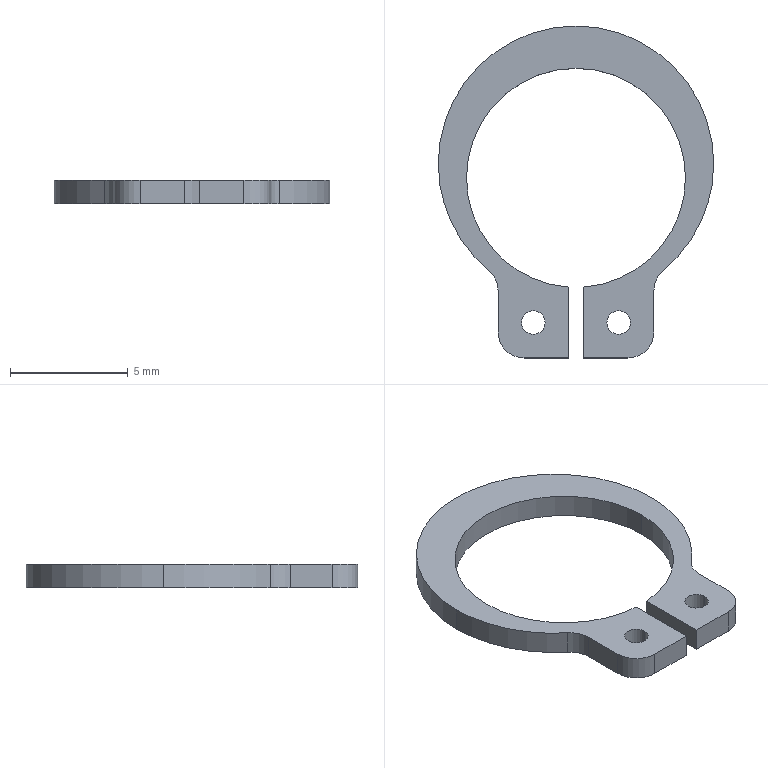Part | NX | features BREP 1 | 1 solid | 22 faces | box 11.7 x 14.1 x 1 mm | volume 53.779 mm3 | cylinder 14 | plane 8 | commonest cylinder face diameters 1 x4 2.207 x4 9.3 x3 11.7 x3
STEP:
#1=CARTESIAN_POINT('',(-2.31,-6.15,0.5));
#2=VERTEX_POINT('',#1);
#3=CARTESIAN_POINT('',(-1.31,-6.15,0.5));
#4=VERTEX_POINT('',#3);
#5=CARTESIAN_POINT('',(-1.81,-6.15,0.5));
#6=DIRECTION('',(0.,0.,1.));
#7=DIRECTION('',(1.,0.,0.));
#8=AXIS2_PLACEMENT_3D('',#5,#6,#7);
#9=CIRCLE('',#8,0.5);
#10=EDGE_CURVE('',#2,#4,#9,.T.);
#11=ORIENTED_EDGE('',*,*,#10,.T.);
#12=CARTESIAN_POINT('',(-1.31,-6.15,-0.5));
#13=VERTEX_POINT('',#12);
#14=CARTESIAN_POINT('',(-1.31,-6.15,0.5));
#15=DIRECTION('',(0.,0.,-1.));
#16=VECTOR('',#15,1000.);
#17=LINE('',#14,#16);
#18=EDGE_CURVE('',#13,#4,#17,.F.);
#19=ORIENTED_EDGE('',*,*,#18,.F.);
#20=CARTESIAN_POINT('',(-2.31,-6.15,-0.5));
#21=VERTEX_POINT('',#20);
#22=CARTESIAN_POINT('',(-1.81,-6.15,-0.5));
#23=DIRECTION('',(0.,0.,1.));
#24=DIRECTION('',(1.,0.,0.));
#25=AXIS2_PLACEMENT_3D('',#22,#23,#24);
#26=CIRCLE('',#25,0.5);
#27=EDGE_CURVE('',#21,#13,#26,.T.);
#28=ORIENTED_EDGE('',*,*,#27,.F.);
#29=CARTESIAN_POINT('',(-2.31,-6.15,0.5));
#30=DIRECTION('',(0.,0.,-1.));
#31=VECTOR('',#30,1000.);
#32=LINE('',#29,#31);
#33=EDGE_CURVE('',#21,#2,#32,.F.);
#34=ORIENTED_EDGE('',*,*,#33,.T.);
#35=EDGE_LOOP('',(#11,#19,#28,#34));
#36=FACE_BOUND('',#35,.T.);
#37=CARTESIAN_POINT('',(-1.81,-6.15,0.5));
#38=DIRECTION('',(0.,0.,-1.));
#39=DIRECTION('',(1.,0.,0.));
#40=AXIS2_PLACEMENT_3D('',#37,#38,#39);
#41=CYLINDRICAL_SURFACE('',#40,0.5);
#42=ADVANCED_FACE('',(#36),#41,.F.);
#43=CARTESIAN_POINT('',(1.31,-6.15,0.5));
#44=VERTEX_POINT('',#43);
#45=CARTESIAN_POINT('',(2.31,-6.15,0.5));
#46=VERTEX_POINT('',#45);
#47=CARTESIAN_POINT('',(1.81,-6.15,0.5));
#48=DIRECTION('',(0.,0.,1.));
#49=DIRECTION('',(1.,0.,0.));
#50=AXIS2_PLACEMENT_3D('',#47,#48,#49);
#51=CIRCLE('',#50,0.5);
#52=EDGE_CURVE('',#44,#46,#51,.T.);
#53=ORIENTED_EDGE('',*,*,#52,.T.);
#54=CARTESIAN_POINT('',(2.31,-6.15,-0.5));
#55=VERTEX_POINT('',#54);
#56=CARTESIAN_POINT('',(2.31,-6.15,0.5));
#57=DIRECTION('',(0.,0.,-1.));
#58=VECTOR('',#57,1000.);
#59=LINE('',#56,#58);
#60=EDGE_CURVE('',#55,#46,#59,.F.);
#61=ORIENTED_EDGE('',*,*,#60,.F.);
#62=CARTESIAN_POINT('',(1.31,-6.15,-0.5));
#63=VERTEX_POINT('',#62);
#64=CARTESIAN_POINT('',(1.81,-6.15,-0.5));
#65=DIRECTION('',(0.,0.,1.));
#66=DIRECTION('',(1.,0.,0.));
#67=AXIS2_PLACEMENT_3D('',#64,#65,#66);
#68=CIRCLE('',#67,0.5);
#69=EDGE_CURVE('',#63,#55,#68,.T.);
#70=ORIENTED_EDGE('',*,*,#69,.F.);
#71=CARTESIAN_POINT('',(1.31,-6.15,0.5));
#72=DIRECTION('',(0.,0.,-1.));
#73=VECTOR('',#72,1000.);
#74=LINE('',#71,#73);
#75=EDGE_CURVE('',#63,#44,#74,.F.);
#76=ORIENTED_EDGE('',*,*,#75,.T.);
#77=EDGE_LOOP('',(#53,#61,#70,#76));
#78=FACE_BOUND('',#77,.T.);
#79=CARTESIAN_POINT('',(1.81,-6.15,0.5));
#80=DIRECTION('',(0.,0.,-1.));
#81=DIRECTION('',(1.,0.,0.));
#82=AXIS2_PLACEMENT_3D('',#79,#80,#81);
#83=CYLINDRICAL_SURFACE('',#82,0.5);
#84=ADVANCED_FACE('',(#78),#83,.F.);
#85=CARTESIAN_POINT('',(4.65,0.,0.5));
#86=VERTEX_POINT('',#85);
#87=CARTESIAN_POINT('',(0.31,-4.64,0.5));
#88=VERTEX_POINT('',#87);
#89=CARTESIAN_POINT('',(0.,0.,0.5));
#90=DIRECTION('',(0.,0.,-1.));
#91=DIRECTION('',(-1.,0.,0.));
#92=AXIS2_PLACEMENT_3D('',#89,#90,#91);
#93=CIRCLE('',#92,4.65);
#94=EDGE_CURVE('',#86,#88,#93,.T.);
#95=ORIENTED_EDGE('',*,*,#94,.F.);
#96=CARTESIAN_POINT('',(4.65,0.,-0.5));
#97=VERTEX_POINT('',#96);
#98=CARTESIAN_POINT('',(4.65,0.,0.5));
#99=DIRECTION('',(0.,0.,-1.));
#100=VECTOR('',#99,1000.);
#101=LINE('',#98,#100);
#102=EDGE_CURVE('',#86,#97,#101,.T.);
#103=ORIENTED_EDGE('',*,*,#102,.T.);
#104=CARTESIAN_POINT('',(0.31,-4.64,-0.5));
#105=VERTEX_POINT('',#104);
#106=CARTESIAN_POINT('',(0.,0.,-0.5));
#107=DIRECTION('',(0.,0.,-1.));
#108=DIRECTION('',(-1.,0.,0.));
#109=AXIS2_PLACEMENT_3D('',#106,#107,#108);
#110=CIRCLE('',#109,4.65);
#111=EDGE_CURVE('',#97,#105,#110,.T.);
#112=ORIENTED_EDGE('',*,*,#111,.T.);
#113=CARTESIAN_POINT('',(0.31,-4.64,0.5));
#114=DIRECTION('',(0.,0.,-1.));
#115=VECTOR('',#114,1000.);
#116=LINE('',#113,#115);
#117=EDGE_CURVE('',#88,#105,#116,.T.);
#118=ORIENTED_EDGE('',*,*,#117,.F.);
#119=EDGE_LOOP('',(#95,#103,#112,#118));
#120=FACE_BOUND('',#119,.T.);
#121=CARTESIAN_POINT('',(0.,0.,0.5));
#122=DIRECTION('',(0.,0.,-1.));
#123=DIRECTION('',(1.,0.,0.));
#124=AXIS2_PLACEMENT_3D('',#121,#122,#123);
#125=CYLINDRICAL_SURFACE('',#124,4.65);
#126=ADVANCED_FACE('',(#120),#125,.F.);
#127=ORIENTED_EDGE('',*,*,#102,.F.);
#128=CARTESIAN_POINT('',(-4.65,0.,0.5));
#129=VERTEX_POINT('',#128);
#130=CARTESIAN_POINT('',(0.,0.,0.5));
#131=DIRECTION('',(0.,0.,-1.));
#132=DIRECTION('',(-1.,0.,0.));
#133=AXIS2_PLACEMENT_3D('',#130,#131,#132);
#134=CIRCLE('',#133,4.65);
#135=EDGE_CURVE('',#129,#86,#134,.T.);
#136=ORIENTED_EDGE('',*,*,#135,.F.);
#137=CARTESIAN_POINT('',(-4.65,0.,-0.5));
#138=VERTEX_POINT('',#137);
#139=CARTESIAN_POINT('',(-4.65,0.,0.5));
#140=DIRECTION('',(0.,0.,-1.));
#141=VECTOR('',#140,1000.);
#142=LINE('',#139,#141);
#143=EDGE_CURVE('',#129,#138,#142,.T.);
#144=ORIENTED_EDGE('',*,*,#143,.T.);
#145=CARTESIAN_POINT('',(0.,0.,-0.5));
#146=DIRECTION('',(0.,0.,-1.));
#147=DIRECTION('',(-1.,0.,0.));
#148=AXIS2_PLACEMENT_3D('',#145,#146,#147);
#149=CIRCLE('',#148,4.65);
#150=EDGE_CURVE('',#138,#97,#149,.T.);
#151=ORIENTED_EDGE('',*,*,#150,.T.);
#152=EDGE_LOOP('',(#127,#136,#144,#151));
#153=FACE_BOUND('',#152,.T.);
#154=CARTESIAN_POINT('',(0.,0.,0.5));
#155=DIRECTION('',(0.,0.,-1.));
#156=DIRECTION('',(1.,0.,0.));
#157=AXIS2_PLACEMENT_3D('',#154,#155,#156);
#158=CYLINDRICAL_SURFACE('',#157,4.65);
#159=ADVANCED_FACE('',(#153),#158,.F.);
#160=CARTESIAN_POINT('',(5.85,0.6,0.5));
#161=VERTEX_POINT('',#160);
#162=CARTESIAN_POINT('',(-5.85,0.6,0.5));
#163=VERTEX_POINT('',#162);
#164=CARTESIAN_POINT('',(0.,0.6,0.5));
#165=DIRECTION('',(0.,0.,1.));
#166=DIRECTION('',(1.,0.,0.));
#167=AXIS2_PLACEMENT_3D('',#164,#165,#166);
#168=CIRCLE('',#167,5.85);
#169=EDGE_CURVE('',#161,#163,#168,.T.);
#170=ORIENTED_EDGE('',*,*,#169,.F.);
#171=CARTESIAN_POINT('',(5.85,0.6,-0.5));
#172=VERTEX_POINT('',#171);
#173=CARTESIAN_POINT('',(5.85,0.6,0.5));
#174=DIRECTION('',(0.,0.,-1.));
#175=VECTOR('',#174,1000.);
#176=LINE('',#173,#175);
#177=EDGE_CURVE('',#161,#172,#176,.T.);
#178=ORIENTED_EDGE('',*,*,#177,.T.);
#179=CARTESIAN_POINT('',(-5.85,0.6,-0.5));
#180=VERTEX_POINT('',#179);
#181=CARTESIAN_POINT('',(0.,0.6,-0.5));
#182=DIRECTION('',(0.,0.,1.));
#183=DIRECTION('',(1.,0.,0.));
#184=AXIS2_PLACEMENT_3D('',#181,#182,#183);
#185=CIRCLE('',#184,5.85);
#186=EDGE_CURVE('',#172,#180,#185,.T.);
#187=ORIENTED_EDGE('',*,*,#186,.T.);
#188=CARTESIAN_POINT('',(-5.85,0.6,0.5));
#189=DIRECTION('',(0.,0.,-1.));
#190=VECTOR('',#189,1000.);
#191=LINE('',#188,#190);
#192=EDGE_CURVE('',#163,#180,#191,.T.);
#193=ORIENTED_EDGE('',*,*,#192,.F.);
#194=EDGE_LOOP('',(#170,#178,#187,#193));
#195=FACE_BOUND('',#194,.T.);
#196=CARTESIAN_POINT('',(0.,0.6,0.5));
#197=DIRECTION('',(0.,0.,-1.));
#198=DIRECTION('',(1.,0.,0.));
#199=AXIS2_PLACEMENT_3D('',#196,#197,#198);
#200=CYLINDRICAL_SURFACE('',#199,5.85);
#201=ADVANCED_FACE('',(#195),#200,.T.);
#202=CARTESIAN_POINT('',(-3.713,-3.921,0.5));
#203=VERTEX_POINT('',#202);
#204=CARTESIAN_POINT('',(0.,0.6,0.5));
#205=DIRECTION('',(0.,0.,1.));
#206=DIRECTION('',(1.,0.,0.));
#207=AXIS2_PLACEMENT_3D('',#204,#205,#206);
#208=CIRCLE('',#207,5.85);
#209=EDGE_CURVE('',#163,#203,#208,.T.);
#210=ORIENTED_EDGE('',*,*,#209,.F.);
#211=ORIENTED_EDGE('',*,*,#192,.T.);
#212=CARTESIAN_POINT('',(-3.713,-3.921,-0.5));
#213=VERTEX_POINT('',#212);
#214=CARTESIAN_POINT('',(0.,0.6,-0.5));
#215=DIRECTION('',(0.,0.,1.));
#216=DIRECTION('',(1.,0.,0.));
#217=AXIS2_PLACEMENT_3D('',#214,#215,#216);
#218=CIRCLE('',#217,5.85);
#219=EDGE_CURVE('',#180,#213,#218,.T.);
#220=ORIENTED_EDGE('',*,*,#219,.T.);
#221=CARTESIAN_POINT('',(-3.713,-3.921,0.5));
#222=DIRECTION('',(0.,0.,-1.));
#223=VECTOR('',#222,1000.);
#224=LINE('',#221,#223);
#225=EDGE_CURVE('',#203,#213,#224,.T.);
#226=ORIENTED_EDGE('',*,*,#225,.F.);
#227=EDGE_LOOP('',(#210,#211,#220,#226));
#228=FACE_BOUND('',#227,.T.);
#229=CARTESIAN_POINT('',(0.,0.6,0.5));
#230=DIRECTION('',(0.,0.,-1.));
#231=DIRECTION('',(1.,0.,0.));
#232=AXIS2_PLACEMENT_3D('',#229,#230,#231);
#233=CYLINDRICAL_SURFACE('',#232,5.85);
#234=ADVANCED_FACE('',(#228),#233,.T.);
#235=CARTESIAN_POINT('',(3.31,-4.773,0.5));
#236=VERTEX_POINT('',#235);
#237=CARTESIAN_POINT('',(3.713,-3.921,0.5));
#238=VERTEX_POINT('',#237);
#239=CARTESIAN_POINT('',(4.413,-4.773,0.5));
#240=DIRECTION('',(0.,0.,-1.));
#241=DIRECTION('',(-1.,0.,0.));
#242=AXIS2_PLACEMENT_3D('',#239,#240,#241);
#243=CIRCLE('',#242,1.103);
#244=EDGE_CURVE('',#236,#238,#243,.T.);
#245=ORIENTED_EDGE('',*,*,#244,.T.);
#246=CARTESIAN_POINT('',(0.,0.6,0.5));
#247=DIRECTION('',(0.,0.,1.));
#248=DIRECTION('',(1.,0.,0.));
#249=AXIS2_PLACEMENT_3D('',#246,#247,#248);
#250=CIRCLE('',#249,5.85);
#251=EDGE_CURVE('',#238,#161,#250,.T.);
#252=ORIENTED_EDGE('',*,*,#251,.T.);
#253=ORIENTED_EDGE('',*,*,#169,.T.);
#254=ORIENTED_EDGE('',*,*,#209,.T.);
#255=CARTESIAN_POINT('',(-3.31,-4.773,0.5));
#256=VERTEX_POINT('',#255);
#257=CARTESIAN_POINT('',(-4.413,-4.773,0.5));
#258=DIRECTION('',(0.,0.,-1.));
#259=DIRECTION('',(-1.,0.,0.));
#260=AXIS2_PLACEMENT_3D('',#257,#258,#259);
#261=CIRCLE('',#260,1.103);
#262=EDGE_CURVE('',#203,#256,#261,.T.);
#263=ORIENTED_EDGE('',*,*,#262,.T.);
#264=CARTESIAN_POINT('',(-3.31,-6.547,0.5));
#265=VERTEX_POINT('',#264);
#266=CARTESIAN_POINT('',(-3.31,-4.773,0.5));
#267=DIRECTION('',(0.,-1.,0.));
#268=VECTOR('',#267,1000.);
#269=LINE('',#266,#268);
#270=EDGE_CURVE('',#256,#265,#269,.T.);
#271=ORIENTED_EDGE('',*,*,#270,.T.);
#272=CARTESIAN_POINT('',(-2.207,-7.65,0.5));
#273=VERTEX_POINT('',#272);
#274=CARTESIAN_POINT('',(-2.207,-6.547,0.5));
#275=DIRECTION('',(0.,0.,1.));
#276=DIRECTION('',(1.,0.,0.));
#277=AXIS2_PLACEMENT_3D('',#274,#275,#276);
#278=CIRCLE('',#277,1.103);
#279=EDGE_CURVE('',#265,#273,#278,.T.);
#280=ORIENTED_EDGE('',*,*,#279,.T.);
#281=CARTESIAN_POINT('',(-0.31,-7.65,0.5));
#282=VERTEX_POINT('',#281);
#283=CARTESIAN_POINT('',(-2.207,-7.65,0.5));
#284=DIRECTION('',(1.,0.,0.));
#285=VECTOR('',#284,1000.);
#286=LINE('',#283,#285);
#287=EDGE_CURVE('',#273,#282,#286,.T.);
#288=ORIENTED_EDGE('',*,*,#287,.T.);
#289=CARTESIAN_POINT('',(-0.31,-4.64,0.5));
#290=VERTEX_POINT('',#289);
#291=CARTESIAN_POINT('',(-0.31,-7.65,0.5));
#292=DIRECTION('',(0.,1.,0.));
#293=VECTOR('',#292,1000.);
#294=LINE('',#291,#293);
#295=EDGE_CURVE('',#282,#290,#294,.T.);
#296=ORIENTED_EDGE('',*,*,#295,.T.);
#297=CARTESIAN_POINT('',(0.,0.,0.5));
#298=DIRECTION('',(0.,0.,-1.));
#299=DIRECTION('',(-1.,0.,0.));
#300=AXIS2_PLACEMENT_3D('',#297,#298,#299);
#301=CIRCLE('',#300,4.65);
#302=EDGE_CURVE('',#290,#129,#301,.T.);
#303=ORIENTED_EDGE('',*,*,#302,.T.);
#304=ORIENTED_EDGE('',*,*,#135,.T.);
#305=ORIENTED_EDGE('',*,*,#94,.T.);
#306=CARTESIAN_POINT('',(0.31,-7.65,0.5));
#307=VERTEX_POINT('',#306);
#308=CARTESIAN_POINT('',(0.31,-4.64,0.5));
#309=DIRECTION('',(0.,-1.,0.));
#310=VECTOR('',#309,1000.);
#311=LINE('',#308,#310);
#312=EDGE_CURVE('',#88,#307,#311,.T.);
#313=ORIENTED_EDGE('',*,*,#312,.T.);
#314=CARTESIAN_POINT('',(2.207,-7.65,0.5));
#315=VERTEX_POINT('',#314);
#316=CARTESIAN_POINT('',(0.31,-7.65,0.5));
#317=DIRECTION('',(1.,0.,0.));
#318=VECTOR('',#317,1000.);
#319=LINE('',#316,#318);
#320=EDGE_CURVE('',#307,#315,#319,.T.);
#321=ORIENTED_EDGE('',*,*,#320,.T.);
#322=CARTESIAN_POINT('',(3.31,-6.547,0.5));
#323=VERTEX_POINT('',#322);
#324=CARTESIAN_POINT('',(2.207,-6.547,0.5));
#325=DIRECTION('',(0.,0.,1.));
#326=DIRECTION('',(1.,0.,0.));
#327=AXIS2_PLACEMENT_3D('',#324,#325,#326);
#328=CIRCLE('',#327,1.103);
#329=EDGE_CURVE('',#315,#323,#328,.T.);
#330=ORIENTED_EDGE('',*,*,#329,.T.);
#331=CARTESIAN_POINT('',(3.31,-6.547,0.5));
#332=DIRECTION('',(0.,1.,0.));
#333=VECTOR('',#332,1000.);
#334=LINE('',#331,#333);
#335=EDGE_CURVE('',#323,#236,#334,.T.);
#336=ORIENTED_EDGE('',*,*,#335,.T.);
#337=EDGE_LOOP('',(#245,#252,#253,#254,#263,#271,#280,#288,#296,#303,#304,#305,#313,#321,#330,#336));
#338=FACE_BOUND('',#337,.T.);
#339=ORIENTED_EDGE('',*,*,#52,.F.);
#340=CARTESIAN_POINT('',(1.81,-6.15,0.5));
#341=DIRECTION('',(0.,0.,1.));
#342=DIRECTION('',(1.,0.,0.));
#343=AXIS2_PLACEMENT_3D('',#340,#341,#342);
#344=CIRCLE('',#343,0.5);
#345=EDGE_CURVE('',#46,#44,#344,.T.);
#346=ORIENTED_EDGE('',*,*,#345,.F.);
#347=EDGE_LOOP('',(#339,#346));
#348=FACE_BOUND('',#347,.T.);
#349=ORIENTED_EDGE('',*,*,#10,.F.);
#350=CARTESIAN_POINT('',(-1.81,-6.15,0.5));
#351=DIRECTION('',(0.,0.,1.));
#352=DIRECTION('',(1.,0.,0.));
#353=AXIS2_PLACEMENT_3D('',#350,#351,#352);
#354=CIRCLE('',#353,0.5);
#355=EDGE_CURVE('',#4,#2,#354,.T.);
#356=ORIENTED_EDGE('',*,*,#355,.F.);
#357=EDGE_LOOP('',(#349,#356));
#358=FACE_BOUND('',#357,.T.);
#359=CARTESIAN_POINT('',(4.413,-4.773,0.5));
#360=DIRECTION('',(0.,0.,-1.));
#361=DIRECTION('',(1.,0.,0.));
#362=AXIS2_PLACEMENT_3D('',#359,#360,#361);
#363=PLANE('',#362);
#364=ADVANCED_FACE('',(#338,#348,#358),#363,.F.);
#365=CARTESIAN_POINT('',(3.31,-4.773,-0.5));
#366=VERTEX_POINT('',#365);
#367=CARTESIAN_POINT('',(3.31,-4.773,0.5));
#368=DIRECTION('',(0.,0.,-1.));
#369=VECTOR('',#368,1000.);
#370=LINE('',#367,#369);
#371=EDGE_CURVE('',#236,#366,#370,.T.);
#372=ORIENTED_EDGE('',*,*,#371,.T.);
#373=CARTESIAN_POINT('',(3.713,-3.921,-0.5));
#374=VERTEX_POINT('',#373);
#375=CARTESIAN_POINT('',(4.413,-4.773,-0.5));
#376=DIRECTION('',(0.,0.,-1.));
#377=DIRECTION('',(-1.,0.,0.));
#378=AXIS2_PLACEMENT_3D('',#375,#376,#377);
#379=CIRCLE('',#378,1.103);
#380=EDGE_CURVE('',#366,#374,#379,.T.);
#381=ORIENTED_EDGE('',*,*,#380,.T.);
#382=CARTESIAN_POINT('',(3.713,-3.921,0.5));
#383=DIRECTION('',(0.,0.,-1.));
#384=VECTOR('',#383,1000.);
#385=LINE('',#382,#384);
#386=EDGE_CURVE('',#238,#374,#385,.T.);
#387=ORIENTED_EDGE('',*,*,#386,.F.);
#388=ORIENTED_EDGE('',*,*,#244,.F.);
#389=EDGE_LOOP('',(#372,#381,#387,#388));
#390=FACE_BOUND('',#389,.T.);
#391=CARTESIAN_POINT('',(4.413,-4.773,0.5));
#392=DIRECTION('',(0.,0.,-1.));
#393=DIRECTION('',(1.,0.,0.));
#394=AXIS2_PLACEMENT_3D('',#391,#392,#393);
#395=CYLINDRICAL_SURFACE('',#394,1.103);
#396=ADVANCED_FACE('',(#390),#395,.F.);
#397=ORIENTED_EDGE('',*,*,#177,.F.);
#398=ORIENTED_EDGE('',*,*,#251,.F.);
#399=ORIENTED_EDGE('',*,*,#386,.T.);
#400=CARTESIAN_POINT('',(0.,0.6,-0.5));
#401=DIRECTION('',(0.,0.,1.));
#402=DIRECTION('',(1.,0.,0.));
#403=AXIS2_PLACEMENT_3D('',#400,#401,#402);
#404=CIRCLE('',#403,5.85);
#405=EDGE_CURVE('',#374,#172,#404,.T.);
#406=ORIENTED_EDGE('',*,*,#405,.T.);
#407=EDGE_LOOP('',(#397,#398,#399,#406));
#408=FACE_BOUND('',#407,.T.);
#409=CARTESIAN_POINT('',(0.,0.6,0.5));
#410=DIRECTION('',(0.,0.,-1.));
#411=DIRECTION('',(1.,0.,0.));
#412=AXIS2_PLACEMENT_3D('',#409,#410,#411);
#413=CYLINDRICAL_SURFACE('',#412,5.85);
#414=ADVANCED_FACE('',(#408),#413,.T.);
#415=ORIENTED_EDGE('',*,*,#225,.T.);
#416=CARTESIAN_POINT('',(-3.31,-4.773,-0.5));
#417=VERTEX_POINT('',#416);
#418=CARTESIAN_POINT('',(-4.413,-4.773,-0.5));
#419=DIRECTION('',(0.,0.,-1.));
#420=DIRECTION('',(-1.,0.,0.));
#421=AXIS2_PLACEMENT_3D('',#418,#419,#420);
#422=CIRCLE('',#421,1.103);
#423=EDGE_CURVE('',#213,#417,#422,.T.);
#424=ORIENTED_EDGE('',*,*,#423,.T.);
#425=CARTESIAN_POINT('',(-3.31,-4.773,0.5));
#426=DIRECTION('',(0.,0.,-1.));
#427=VECTOR('',#426,1000.);
#428=LINE('',#425,#427);
#429=EDGE_CURVE('',#256,#417,#428,.T.);
#430=ORIENTED_EDGE('',*,*,#429,.F.);
#431=ORIENTED_EDGE('',*,*,#262,.F.);
#432=EDGE_LOOP('',(#415,#424,#430,#431));
#433=FACE_BOUND('',#432,.T.);
#434=CARTESIAN_POINT('',(-4.413,-4.773,0.5));
#435=DIRECTION('',(0.,0.,-1.));
#436=DIRECTION('',(1.,0.,0.));
#437=AXIS2_PLACEMENT_3D('',#434,#435,#436);
#438=CYLINDRICAL_SURFACE('',#437,1.103);
#439=ADVANCED_FACE('',(#433),#438,.F.);
#440=ORIENTED_EDGE('',*,*,#429,.T.);
#441=CARTESIAN_POINT('',(-3.31,-6.547,-0.5));
#442=VERTEX_POINT('',#441);
#443=CARTESIAN_POINT('',(-3.31,-4.773,-0.5));
#444=DIRECTION('',(0.,-1.,0.));
#445=VECTOR('',#444,1000.);
#446=LINE('',#443,#445);
#447=EDGE_CURVE('',#417,#442,#446,.T.);
#448=ORIENTED_EDGE('',*,*,#447,.T.);
#449=CARTESIAN_POINT('',(-3.31,-6.547,0.5));
#450=DIRECTION('',(0.,0.,-1.));
#451=VECTOR('',#450,1000.);
#452=LINE('',#449,#451);
#453=EDGE_CURVE('',#265,#442,#452,.T.);
#454=ORIENTED_EDGE('',*,*,#453,.F.);
#455=ORIENTED_EDGE('',*,*,#270,.F.);
#456=EDGE_LOOP('',(#440,#448,#454,#455));
#457=FACE_BOUND('',#456,.T.);
#458=CARTESIAN_POINT('',(-3.31,-4.773,0.5));
#459=DIRECTION('',(1.,0.,0.));
#460=DIRECTION('',(0.,0.,1.));
#461=AXIS2_PLACEMENT_3D('',#458,#459,#460);
#462=PLANE('',#461);
#463=ADVANCED_FACE('',(#457),#462,.F.);
#464=ORIENTED_EDGE('',*,*,#453,.T.);
#465=CARTESIAN_POINT('',(-2.207,-7.65,-0.5));
#466=VERTEX_POINT('',#465);
#467=CARTESIAN_POINT('',(-2.207,-6.547,-0.5));
#468=DIRECTION('',(0.,0.,1.));
#469=DIRECTION('',(1.,0.,0.));
#470=AXIS2_PLACEMENT_3D('',#467,#468,#469);
#471=CIRCLE('',#470,1.103);
#472=EDGE_CURVE('',#442,#466,#471,.T.);
#473=ORIENTED_EDGE('',*,*,#472,.T.);
#474=CARTESIAN_POINT('',(-2.207,-7.65,0.5));
#475=DIRECTION('',(0.,0.,-1.));
#476=VECTOR('',#475,1000.);
#477=LINE('',#474,#476);
#478=EDGE_CURVE('',#273,#466,#477,.T.);
#479=ORIENTED_EDGE('',*,*,#478,.F.);
#480=ORIENTED_EDGE('',*,*,#279,.F.);
#481=EDGE_LOOP('',(#464,#473,#479,#480));
#482=FACE_BOUND('',#481,.T.);
#483=CARTESIAN_POINT('',(-2.207,-6.547,0.5));
#484=DIRECTION('',(0.,0.,-1.));
#485=DIRECTION('',(1.,0.,0.));
#486=AXIS2_PLACEMENT_3D('',#483,#484,#485);
#487=CYLINDRICAL_SURFACE('',#486,1.103);
#488=ADVANCED_FACE('',(#482),#487,.T.);
#489=ORIENTED_EDGE('',*,*,#478,.T.);
#490=CARTESIAN_POINT('',(-0.31,-7.65,-0.5));
#491=VERTEX_POINT('',#490);
#492=CARTESIAN_POINT('',(-2.207,-7.65,-0.5));
#493=DIRECTION('',(1.,0.,0.));
#494=VECTOR('',#493,1000.);
#495=LINE('',#492,#494);
#496=EDGE_CURVE('',#466,#491,#495,.T.);
#497=ORIENTED_EDGE('',*,*,#496,.T.);
#498=CARTESIAN_POINT('',(-0.31,-7.65,0.5));
#499=DIRECTION('',(0.,0.,-1.));
#500=VECTOR('',#499,1000.);
#501=LINE('',#498,#500);
#502=EDGE_CURVE('',#282,#491,#501,.T.);
#503=ORIENTED_EDGE('',*,*,#502,.F.);
#504=ORIENTED_EDGE('',*,*,#287,.F.);
#505=EDGE_LOOP('',(#489,#497,#503,#504));
#506=FACE_BOUND('',#505,.T.);
#507=CARTESIAN_POINT('',(-2.207,-7.65,0.5));
#508=DIRECTION('',(0.,1.,0.));
#509=DIRECTION('',(0.,0.,-1.));
#510=AXIS2_PLACEMENT_3D('',#507,#508,#509);
#511=PLANE('',#510);
#512=ADVANCED_FACE('',(#506),#511,.F.);
#513=ORIENTED_EDGE('',*,*,#502,.T.);
#514=CARTESIAN_POINT('',(-0.31,-4.64,-0.5));
#515=VERTEX_POINT('',#514);
#516=CARTESIAN_POINT('',(-0.31,-7.65,-0.5));
#517=DIRECTION('',(0.,1.,0.));
#518=VECTOR('',#517,1000.);
#519=LINE('',#516,#518);
#520=EDGE_CURVE('',#491,#515,#519,.T.);
#521=ORIENTED_EDGE('',*,*,#520,.T.);
#522=CARTESIAN_POINT('',(-0.31,-4.64,0.5));
#523=DIRECTION('',(0.,0.,-1.));
#524=VECTOR('',#523,1000.);
#525=LINE('',#522,#524);
#526=EDGE_CURVE('',#290,#515,#525,.T.);
#527=ORIENTED_EDGE('',*,*,#526,.F.);
#528=ORIENTED_EDGE('',*,*,#295,.F.);
#529=EDGE_LOOP('',(#513,#521,#527,#528));
#530=FACE_BOUND('',#529,.T.);
#531=CARTESIAN_POINT('',(-0.31,-7.65,0.5));
#532=DIRECTION('',(-1.,0.,0.));
#533=DIRECTION('',(0.,0.,-1.));
#534=AXIS2_PLACEMENT_3D('',#531,#532,#533);
#535=PLANE('',#534);
#536=ADVANCED_FACE('',(#530),#535,.F.);
#537=ORIENTED_EDGE('',*,*,#143,.F.);
#538=ORIENTED_EDGE('',*,*,#302,.F.);
#539=ORIENTED_EDGE('',*,*,#526,.T.);
#540=CARTESIAN_POINT('',(0.,0.,-0.5));
#541=DIRECTION('',(0.,0.,-1.));
#542=DIRECTION('',(-1.,0.,0.));
#543=AXIS2_PLACEMENT_3D('',#540,#541,#542);
#544=CIRCLE('',#543,4.65);
#545=EDGE_CURVE('',#515,#138,#544,.T.);
#546=ORIENTED_EDGE('',*,*,#545,.T.);
#547=EDGE_LOOP('',(#537,#538,#539,#546));
#548=FACE_BOUND('',#547,.T.);
#549=CARTESIAN_POINT('',(0.,0.,0.5));
#550=DIRECTION('',(0.,0.,-1.));
#551=DIRECTION('',(1.,0.,0.));
#552=AXIS2_PLACEMENT_3D('',#549,#550,#551);
#553=CYLINDRICAL_SURFACE('',#552,4.65);
#554=ADVANCED_FACE('',(#548),#553,.F.);
#555=ORIENTED_EDGE('',*,*,#117,.T.);
#556=CARTESIAN_POINT('',(0.31,-7.65,-0.5));
#557=VERTEX_POINT('',#556);
#558=CARTESIAN_POINT('',(0.31,-4.64,-0.5));
#559=DIRECTION('',(0.,-1.,0.));
#560=VECTOR('',#559,1000.);
#561=LINE('',#558,#560);
#562=EDGE_CURVE('',#105,#557,#561,.T.);
#563=ORIENTED_EDGE('',*,*,#562,.T.);
#564=CARTESIAN_POINT('',(0.31,-7.65,0.5));
#565=DIRECTION('',(0.,0.,-1.));
#566=VECTOR('',#565,1000.);
#567=LINE('',#564,#566);
#568=EDGE_CURVE('',#307,#557,#567,.T.);
#569=ORIENTED_EDGE('',*,*,#568,.F.);
#570=ORIENTED_EDGE('',*,*,#312,.F.);
#571=EDGE_LOOP('',(#555,#563,#569,#570));
#572=FACE_BOUND('',#571,.T.);
#573=CARTESIAN_POINT('',(0.31,-4.64,0.5));
#574=DIRECTION('',(1.,0.,0.));
#575=DIRECTION('',(0.,0.,1.));
#576=AXIS2_PLACEMENT_3D('',#573,#574,#575);
#577=PLANE('',#576);
#578=ADVANCED_FACE('',(#572),#577,.F.);
#579=ORIENTED_EDGE('',*,*,#568,.T.);
#580=CARTESIAN_POINT('',(2.207,-7.65,-0.5));
#581=VERTEX_POINT('',#580);
#582=CARTESIAN_POINT('',(0.31,-7.65,-0.5));
#583=DIRECTION('',(1.,0.,0.));
#584=VECTOR('',#583,1000.);
#585=LINE('',#582,#584);
#586=EDGE_CURVE('',#557,#581,#585,.T.);
#587=ORIENTED_EDGE('',*,*,#586,.T.);
#588=CARTESIAN_POINT('',(2.207,-7.65,0.5));
#589=DIRECTION('',(0.,0.,-1.));
#590=VECTOR('',#589,1000.);
#591=LINE('',#588,#590);
#592=EDGE_CURVE('',#315,#581,#591,.T.);
#593=ORIENTED_EDGE('',*,*,#592,.F.);
#594=ORIENTED_EDGE('',*,*,#320,.F.);
#595=EDGE_LOOP('',(#579,#587,#593,#594));
#596=FACE_BOUND('',#595,.T.);
#597=CARTESIAN_POINT('',(0.31,-7.65,0.5));
#598=DIRECTION('',(0.,1.,0.));
#599=DIRECTION('',(0.,0.,-1.));
#600=AXIS2_PLACEMENT_3D('',#597,#598,#599);
#601=PLANE('',#600);
#602=ADVANCED_FACE('',(#596),#601,.F.);
#603=ORIENTED_EDGE('',*,*,#592,.T.);
#604=CARTESIAN_POINT('',(3.31,-6.547,-0.5));
#605=VERTEX_POINT('',#604);
#606=CARTESIAN_POINT('',(2.207,-6.547,-0.5));
#607=DIRECTION('',(0.,0.,1.));
#608=DIRECTION('',(1.,0.,0.));
#609=AXIS2_PLACEMENT_3D('',#606,#607,#608);
#610=CIRCLE('',#609,1.103);
#611=EDGE_CURVE('',#581,#605,#610,.T.);
#612=ORIENTED_EDGE('',*,*,#611,.T.);
#613=CARTESIAN_POINT('',(3.31,-6.547,0.5));
#614=DIRECTION('',(0.,0.,-1.));
#615=VECTOR('',#614,1000.);
#616=LINE('',#613,#615);
#617=EDGE_CURVE('',#323,#605,#616,.T.);
#618=ORIENTED_EDGE('',*,*,#617,.F.);
#619=ORIENTED_EDGE('',*,*,#329,.F.);
#620=EDGE_LOOP('',(#603,#612,#618,#619));
#621=FACE_BOUND('',#620,.T.);
#622=CARTESIAN_POINT('',(2.207,-6.547,0.5));
#623=DIRECTION('',(0.,0.,-1.));
#624=DIRECTION('',(1.,0.,0.));
#625=AXIS2_PLACEMENT_3D('',#622,#623,#624);
#626=CYLINDRICAL_SURFACE('',#625,1.103);
#627=ADVANCED_FACE('',(#621),#626,.T.);
#628=ORIENTED_EDGE('',*,*,#617,.T.);
#629=CARTESIAN_POINT('',(3.31,-6.547,-0.5));
#630=DIRECTION('',(0.,1.,0.));
#631=VECTOR('',#630,1000.);
#632=LINE('',#629,#631);
#633=EDGE_CURVE('',#605,#366,#632,.T.);
#634=ORIENTED_EDGE('',*,*,#633,.T.);
#635=ORIENTED_EDGE('',*,*,#371,.F.);
#636=ORIENTED_EDGE('',*,*,#335,.F.);
#637=EDGE_LOOP('',(#628,#634,#635,#636));
#638=FACE_BOUND('',#637,.T.);
#639=CARTESIAN_POINT('',(3.31,-6.547,0.5));
#640=DIRECTION('',(-1.,0.,0.));
#641=DIRECTION('',(0.,0.,-1.));
#642=AXIS2_PLACEMENT_3D('',#639,#640,#641);
#643=PLANE('',#642);
#644=ADVANCED_FACE('',(#638),#643,.F.);
#645=ORIENTED_EDGE('',*,*,#60,.T.);
#646=ORIENTED_EDGE('',*,*,#345,.T.);
#647=ORIENTED_EDGE('',*,*,#75,.F.);
#648=CARTESIAN_POINT('',(1.81,-6.15,-0.5));
#649=DIRECTION('',(0.,0.,1.));
#650=DIRECTION('',(1.,0.,0.));
#651=AXIS2_PLACEMENT_3D('',#648,#649,#650);
#652=CIRCLE('',#651,0.5);
#653=EDGE_CURVE('',#55,#63,#652,.T.);
#654=ORIENTED_EDGE('',*,*,#653,.F.);
#655=EDGE_LOOP('',(#645,#646,#647,#654));
#656=FACE_BOUND('',#655,.T.);
#657=CARTESIAN_POINT('',(1.81,-6.15,0.5));
#658=DIRECTION('',(0.,0.,-1.));
#659=DIRECTION('',(1.,0.,0.));
#660=AXIS2_PLACEMENT_3D('',#657,#658,#659);
#661=CYLINDRICAL_SURFACE('',#660,0.5);
#662=ADVANCED_FACE('',(#656),#661,.F.);
#663=ORIENTED_EDGE('',*,*,#18,.T.);
#664=ORIENTED_EDGE('',*,*,#355,.T.);
#665=ORIENTED_EDGE('',*,*,#33,.F.);
#666=CARTESIAN_POINT('',(-1.81,-6.15,-0.5));
#667=DIRECTION('',(0.,0.,1.));
#668=DIRECTION('',(1.,0.,0.));
#669=AXIS2_PLACEMENT_3D('',#666,#667,#668);
#670=CIRCLE('',#669,0.5);
#671=EDGE_CURVE('',#13,#21,#670,.T.);
#672=ORIENTED_EDGE('',*,*,#671,.F.);
#673=EDGE_LOOP('',(#663,#664,#665,#672));
#674=FACE_BOUND('',#673,.T.);
#675=CARTESIAN_POINT('',(-1.81,-6.15,0.5));
#676=DIRECTION('',(0.,0.,-1.));
#677=DIRECTION('',(1.,0.,0.));
#678=AXIS2_PLACEMENT_3D('',#675,#676,#677);
#679=CYLINDRICAL_SURFACE('',#678,0.5);
#680=ADVANCED_FACE('',(#674),#679,.F.);
#681=ORIENTED_EDGE('',*,*,#27,.T.);
#682=ORIENTED_EDGE('',*,*,#671,.T.);
#683=EDGE_LOOP('',(#681,#682));
#684=FACE_BOUND('',#683,.T.);
#685=ORIENTED_EDGE('',*,*,#69,.T.);
#686=ORIENTED_EDGE('',*,*,#653,.T.);
#687=EDGE_LOOP('',(#685,#686));
#688=FACE_BOUND('',#687,.T.);
#689=ORIENTED_EDGE('',*,*,#380,.F.);
#690=ORIENTED_EDGE('',*,*,#633,.F.);
#691=ORIENTED_EDGE('',*,*,#611,.F.);
#692=ORIENTED_EDGE('',*,*,#586,.F.);
#693=ORIENTED_EDGE('',*,*,#562,.F.);
#694=ORIENTED_EDGE('',*,*,#111,.F.);
#695=ORIENTED_EDGE('',*,*,#150,.F.);
#696=ORIENTED_EDGE('',*,*,#545,.F.);
#697=ORIENTED_EDGE('',*,*,#520,.F.);
#698=ORIENTED_EDGE('',*,*,#496,.F.);
#699=ORIENTED_EDGE('',*,*,#472,.F.);
#700=ORIENTED_EDGE('',*,*,#447,.F.);
#701=ORIENTED_EDGE('',*,*,#423,.F.);
#702=ORIENTED_EDGE('',*,*,#219,.F.);
#703=ORIENTED_EDGE('',*,*,#186,.F.);
#704=ORIENTED_EDGE('',*,*,#405,.F.);
#705=EDGE_LOOP('',(#689,#690,#691,#692,#693,#694,#695,#696,#697,#698,#699,#700,#701,#702,#703,#704));
#706=FACE_BOUND('',#705,.T.);
#707=CARTESIAN_POINT('',(4.413,-4.773,-0.5));
#708=DIRECTION('',(0.,0.,-1.));
#709=DIRECTION('',(1.,0.,0.));
#710=AXIS2_PLACEMENT_3D('',#707,#708,#709);
#711=PLANE('',#710);
#712=ADVANCED_FACE('',(#684,#688,#706),#711,.T.);
#713=CLOSED_SHELL('',(#42,#84,#126,#159,#201,#234,#364,#396,#414,#439,#463,#488,#512,#536,#554,#578,#602,#627,#644,#662,#680,#712));
#714=MANIFOLD_SOLID_BREP('',#713);
#715=(LENGTH_UNIT()NAMED_UNIT(*)SI_UNIT(.MILLI.,.METRE.));
#716=UNCERTAINTY_MEASURE_WITH_UNIT(LENGTH_MEASURE(0.00001),#715,'','');
#717=(NAMED_UNIT(*)PLANE_ANGLE_UNIT()SI_UNIT($,.RADIAN.));
#718=(NAMED_UNIT(*)SI_UNIT($,.STERADIAN.)SOLID_ANGLE_UNIT());
#719=(GEOMETRIC_REPRESENTATION_CONTEXT(3)GLOBAL_UNCERTAINTY_ASSIGNED_CONTEXT((#716))GLOBAL_UNIT_ASSIGNED_CONTEXT((#715,#717,#718))REPRESENTATION_CONTEXT('',''));
#720=ADVANCED_BREP_SHAPE_REPRESENTATION('',(#714),#719);